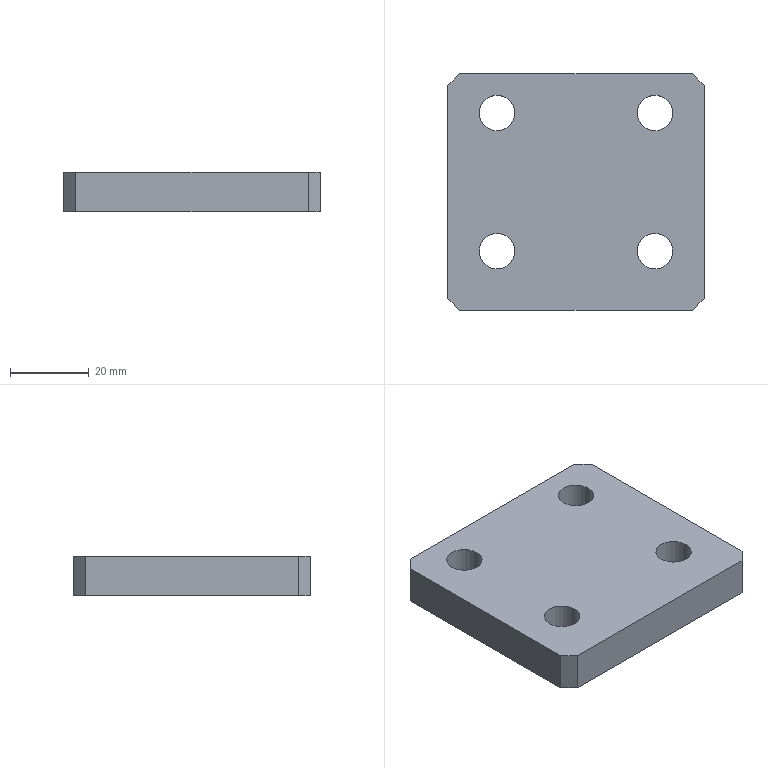Part | SolidWorks | features BaseBody 1 | 1 solid | 18 faces | box 65 x 60 x 10 mm | volume 36275 mm3 | plane 10 | cylinder 8 | commonest cylinder face diameters 9 x8
STEP:
#1=CARTESIAN_POINT('',(24.5,-15.,10.));
#2=VERTEX_POINT('',#1);
#3=CARTESIAN_POINT('',(15.5,-15.,10.));
#4=VERTEX_POINT('',#3);
#5=CARTESIAN_POINT('',(20.,-15.,10.));
#6=DIRECTION('',(0.,0.,-1.));
#7=DIRECTION('',(-1.,0.,0.));
#8=AXIS2_PLACEMENT_3D('',#5,#6,#7);
#9=CIRCLE('',#8,4.5);
#10=EDGE_CURVE('',#2,#4,#9,.T.);
#11=ORIENTED_EDGE('',*,*,#10,.F.);
#12=CARTESIAN_POINT('',(24.5,-15.,0.));
#13=VERTEX_POINT('',#12);
#14=CARTESIAN_POINT('',(24.5,-15.,0.));
#15=DIRECTION('',(0.,0.,-1.));
#16=VECTOR('',#15,1000.);
#17=LINE('',#14,#16);
#18=EDGE_CURVE('',#2,#13,#17,.T.);
#19=ORIENTED_EDGE('',*,*,#18,.T.);
#20=CARTESIAN_POINT('',(15.5,-15.,0.));
#21=VERTEX_POINT('',#20);
#22=CARTESIAN_POINT('',(20.,-15.,0.));
#23=DIRECTION('',(0.,0.,-1.));
#24=DIRECTION('',(-1.,0.,0.));
#25=AXIS2_PLACEMENT_3D('',#22,#23,#24);
#26=CIRCLE('',#25,4.5);
#27=EDGE_CURVE('',#13,#21,#26,.T.);
#28=ORIENTED_EDGE('',*,*,#27,.T.);
#29=CARTESIAN_POINT('',(15.5,-15.,0.));
#30=DIRECTION('',(0.,0.,-1.));
#31=VECTOR('',#30,1000.);
#32=LINE('',#29,#31);
#33=EDGE_CURVE('',#4,#21,#32,.T.);
#34=ORIENTED_EDGE('',*,*,#33,.F.);
#35=EDGE_LOOP('',(#11,#19,#28,#34));
#36=FACE_OUTER_BOUND('',#35,.T.);
#37=CARTESIAN_POINT('',(20.,-15.,0.));
#38=DIRECTION('',(0.,0.,-1.));
#39=DIRECTION('',(-1.,0.,0.));
#40=AXIS2_PLACEMENT_3D('',#37,#38,#39);
#41=CYLINDRICAL_SURFACE('',#40,4.5);
#42=ADVANCED_FACE('',(#36),#41,.F.);
#43=CARTESIAN_POINT('',(-15.5,-15.,10.));
#44=VERTEX_POINT('',#43);
#45=CARTESIAN_POINT('',(-24.5,-15.,10.));
#46=VERTEX_POINT('',#45);
#47=CARTESIAN_POINT('',(-20.,-15.,10.));
#48=DIRECTION('',(0.,0.,-1.));
#49=DIRECTION('',(-1.,0.,0.));
#50=AXIS2_PLACEMENT_3D('',#47,#48,#49);
#51=CIRCLE('',#50,4.5);
#52=EDGE_CURVE('',#44,#46,#51,.T.);
#53=ORIENTED_EDGE('',*,*,#52,.F.);
#54=CARTESIAN_POINT('',(-15.5,-15.,0.));
#55=VERTEX_POINT('',#54);
#56=CARTESIAN_POINT('',(-15.5,-15.,0.));
#57=DIRECTION('',(0.,0.,-1.));
#58=VECTOR('',#57,1000.);
#59=LINE('',#56,#58);
#60=EDGE_CURVE('',#44,#55,#59,.T.);
#61=ORIENTED_EDGE('',*,*,#60,.T.);
#62=CARTESIAN_POINT('',(-24.5,-15.,0.));
#63=VERTEX_POINT('',#62);
#64=CARTESIAN_POINT('',(-20.,-15.,0.));
#65=DIRECTION('',(0.,0.,-1.));
#66=DIRECTION('',(-1.,0.,0.));
#67=AXIS2_PLACEMENT_3D('',#64,#65,#66);
#68=CIRCLE('',#67,4.5);
#69=EDGE_CURVE('',#55,#63,#68,.T.);
#70=ORIENTED_EDGE('',*,*,#69,.T.);
#71=CARTESIAN_POINT('',(-24.5,-15.,0.));
#72=DIRECTION('',(0.,0.,-1.));
#73=VECTOR('',#72,1000.);
#74=LINE('',#71,#73);
#75=EDGE_CURVE('',#46,#63,#74,.T.);
#76=ORIENTED_EDGE('',*,*,#75,.F.);
#77=EDGE_LOOP('',(#53,#61,#70,#76));
#78=FACE_OUTER_BOUND('',#77,.T.);
#79=CARTESIAN_POINT('',(-20.,-15.,0.));
#80=DIRECTION('',(0.,0.,-1.));
#81=DIRECTION('',(-1.,0.,0.));
#82=AXIS2_PLACEMENT_3D('',#79,#80,#81);
#83=CYLINDRICAL_SURFACE('',#82,4.5);
#84=ADVANCED_FACE('',(#78),#83,.F.);
#85=CARTESIAN_POINT('',(24.5,20.,10.));
#86=VERTEX_POINT('',#85);
#87=CARTESIAN_POINT('',(15.5,20.,10.));
#88=VERTEX_POINT('',#87);
#89=CARTESIAN_POINT('',(20.,20.,10.));
#90=DIRECTION('',(0.,0.,-1.));
#91=DIRECTION('',(-1.,0.,0.));
#92=AXIS2_PLACEMENT_3D('',#89,#90,#91);
#93=CIRCLE('',#92,4.5);
#94=EDGE_CURVE('',#86,#88,#93,.T.);
#95=ORIENTED_EDGE('',*,*,#94,.F.);
#96=CARTESIAN_POINT('',(24.5,20.,0.));
#97=VERTEX_POINT('',#96);
#98=CARTESIAN_POINT('',(24.5,20.,0.));
#99=DIRECTION('',(0.,0.,-1.));
#100=VECTOR('',#99,1000.);
#101=LINE('',#98,#100);
#102=EDGE_CURVE('',#86,#97,#101,.T.);
#103=ORIENTED_EDGE('',*,*,#102,.T.);
#104=CARTESIAN_POINT('',(15.5,20.,0.));
#105=VERTEX_POINT('',#104);
#106=CARTESIAN_POINT('',(20.,20.,0.));
#107=DIRECTION('',(0.,0.,-1.));
#108=DIRECTION('',(-1.,0.,0.));
#109=AXIS2_PLACEMENT_3D('',#106,#107,#108);
#110=CIRCLE('',#109,4.5);
#111=EDGE_CURVE('',#97,#105,#110,.T.);
#112=ORIENTED_EDGE('',*,*,#111,.T.);
#113=CARTESIAN_POINT('',(15.5,20.,0.));
#114=DIRECTION('',(0.,0.,-1.));
#115=VECTOR('',#114,1000.);
#116=LINE('',#113,#115);
#117=EDGE_CURVE('',#88,#105,#116,.T.);
#118=ORIENTED_EDGE('',*,*,#117,.F.);
#119=EDGE_LOOP('',(#95,#103,#112,#118));
#120=FACE_OUTER_BOUND('',#119,.T.);
#121=CARTESIAN_POINT('',(20.,20.,0.));
#122=DIRECTION('',(0.,0.,-1.));
#123=DIRECTION('',(-1.,0.,0.));
#124=AXIS2_PLACEMENT_3D('',#121,#122,#123);
#125=CYLINDRICAL_SURFACE('',#124,4.5);
#126=ADVANCED_FACE('',(#120),#125,.F.);
#127=CARTESIAN_POINT('',(-15.5,20.,10.));
#128=VERTEX_POINT('',#127);
#129=CARTESIAN_POINT('',(-24.5,20.,10.));
#130=VERTEX_POINT('',#129);
#131=CARTESIAN_POINT('',(-20.,20.,10.));
#132=DIRECTION('',(0.,0.,-1.));
#133=DIRECTION('',(-1.,0.,0.));
#134=AXIS2_PLACEMENT_3D('',#131,#132,#133);
#135=CIRCLE('',#134,4.5);
#136=EDGE_CURVE('',#128,#130,#135,.T.);
#137=ORIENTED_EDGE('',*,*,#136,.F.);
#138=CARTESIAN_POINT('',(-15.5,20.,0.));
#139=VERTEX_POINT('',#138);
#140=CARTESIAN_POINT('',(-15.5,20.,0.));
#141=DIRECTION('',(0.,0.,-1.));
#142=VECTOR('',#141,1000.);
#143=LINE('',#140,#142);
#144=EDGE_CURVE('',#128,#139,#143,.T.);
#145=ORIENTED_EDGE('',*,*,#144,.T.);
#146=CARTESIAN_POINT('',(-24.5,20.,0.));
#147=VERTEX_POINT('',#146);
#148=CARTESIAN_POINT('',(-20.,20.,0.));
#149=DIRECTION('',(0.,0.,-1.));
#150=DIRECTION('',(-1.,0.,0.));
#151=AXIS2_PLACEMENT_3D('',#148,#149,#150);
#152=CIRCLE('',#151,4.5);
#153=EDGE_CURVE('',#139,#147,#152,.T.);
#154=ORIENTED_EDGE('',*,*,#153,.T.);
#155=CARTESIAN_POINT('',(-24.5,20.,0.));
#156=DIRECTION('',(0.,0.,-1.));
#157=VECTOR('',#156,1000.);
#158=LINE('',#155,#157);
#159=EDGE_CURVE('',#130,#147,#158,.T.);
#160=ORIENTED_EDGE('',*,*,#159,.F.);
#161=EDGE_LOOP('',(#137,#145,#154,#160));
#162=FACE_OUTER_BOUND('',#161,.T.);
#163=CARTESIAN_POINT('',(-20.,20.,0.));
#164=DIRECTION('',(0.,0.,-1.));
#165=DIRECTION('',(-1.,0.,0.));
#166=AXIS2_PLACEMENT_3D('',#163,#164,#165);
#167=CYLINDRICAL_SURFACE('',#166,4.5);
#168=ADVANCED_FACE('',(#162),#167,.F.);
#169=CARTESIAN_POINT('',(-32.5,27.,0.));
#170=VERTEX_POINT('',#169);
#171=CARTESIAN_POINT('',(-32.5,-27.,0.));
#172=VERTEX_POINT('',#171);
#173=CARTESIAN_POINT('',(-32.5,30.,0.));
#174=DIRECTION('',(0.,-1.,0.));
#175=VECTOR('',#174,1000.);
#176=LINE('',#173,#175);
#177=EDGE_CURVE('',#170,#172,#176,.T.);
#178=ORIENTED_EDGE('',*,*,#177,.T.);
#179=CARTESIAN_POINT('',(-32.5,-27.,10.));
#180=VERTEX_POINT('',#179);
#181=CARTESIAN_POINT('',(-32.5,-27.,10.));
#182=DIRECTION('',(0.,0.,1.));
#183=VECTOR('',#182,1000.);
#184=LINE('',#181,#183);
#185=EDGE_CURVE('',#172,#180,#184,.T.);
#186=ORIENTED_EDGE('',*,*,#185,.T.);
#187=CARTESIAN_POINT('',(-32.5,27.,10.));
#188=VERTEX_POINT('',#187);
#189=CARTESIAN_POINT('',(-32.5,30.,10.));
#190=DIRECTION('',(0.,-1.,0.));
#191=VECTOR('',#190,1000.);
#192=LINE('',#189,#191);
#193=EDGE_CURVE('',#188,#180,#192,.T.);
#194=ORIENTED_EDGE('',*,*,#193,.F.);
#195=CARTESIAN_POINT('',(-32.5,27.,10.));
#196=DIRECTION('',(0.,0.,-1.));
#197=VECTOR('',#196,1000.);
#198=LINE('',#195,#197);
#199=EDGE_CURVE('',#188,#170,#198,.T.);
#200=ORIENTED_EDGE('',*,*,#199,.T.);
#201=EDGE_LOOP('',(#178,#186,#194,#200));
#202=FACE_OUTER_BOUND('',#201,.T.);
#203=CARTESIAN_POINT('',(-32.5,30.,10.));
#204=DIRECTION('',(1.,0.,0.));
#205=DIRECTION('',(0.,1.,0.));
#206=AXIS2_PLACEMENT_3D('',#203,#204,#205);
#207=PLANE('',#206);
#208=ADVANCED_FACE('',(#202),#207,.F.);
#209=CARTESIAN_POINT('',(-29.5,-30.,10.));
#210=VERTEX_POINT('',#209);
#211=CARTESIAN_POINT('',(29.5,-30.,10.));
#212=VERTEX_POINT('',#211);
#213=CARTESIAN_POINT('',(32.5,-30.,10.));
#214=DIRECTION('',(1.,0.,0.));
#215=VECTOR('',#214,1000.);
#216=LINE('',#213,#215);
#217=EDGE_CURVE('',#210,#212,#216,.T.);
#218=ORIENTED_EDGE('',*,*,#217,.F.);
#219=CARTESIAN_POINT('',(-29.5,-30.,0.));
#220=VERTEX_POINT('',#219);
#221=CARTESIAN_POINT('',(-29.5,-30.,10.));
#222=DIRECTION('',(0.,0.,-1.));
#223=VECTOR('',#222,1000.);
#224=LINE('',#221,#223);
#225=EDGE_CURVE('',#210,#220,#224,.T.);
#226=ORIENTED_EDGE('',*,*,#225,.T.);
#227=CARTESIAN_POINT('',(29.5,-30.,0.));
#228=VERTEX_POINT('',#227);
#229=CARTESIAN_POINT('',(32.5,-30.,0.));
#230=DIRECTION('',(1.,0.,0.));
#231=VECTOR('',#230,1000.);
#232=LINE('',#229,#231);
#233=EDGE_CURVE('',#220,#228,#232,.T.);
#234=ORIENTED_EDGE('',*,*,#233,.T.);
#235=CARTESIAN_POINT('',(29.5,-30.,10.));
#236=DIRECTION('',(0.,0.,1.));
#237=VECTOR('',#236,1000.);
#238=LINE('',#235,#237);
#239=EDGE_CURVE('',#228,#212,#238,.T.);
#240=ORIENTED_EDGE('',*,*,#239,.T.);
#241=EDGE_LOOP('',(#218,#226,#234,#240));
#242=FACE_OUTER_BOUND('',#241,.T.);
#243=CARTESIAN_POINT('',(32.5,-30.,10.));
#244=DIRECTION('',(0.,1.,0.));
#245=DIRECTION('',(-1.,0.,0.));
#246=AXIS2_PLACEMENT_3D('',#243,#244,#245);
#247=PLANE('',#246);
#248=ADVANCED_FACE('',(#242),#247,.F.);
#249=CARTESIAN_POINT('',(32.5,-27.,10.));
#250=VERTEX_POINT('',#249);
#251=CARTESIAN_POINT('',(32.5,27.,10.));
#252=VERTEX_POINT('',#251);
#253=CARTESIAN_POINT('',(32.5,30.,10.));
#254=DIRECTION('',(0.,1.,0.));
#255=VECTOR('',#254,1000.);
#256=LINE('',#253,#255);
#257=EDGE_CURVE('',#250,#252,#256,.T.);
#258=ORIENTED_EDGE('',*,*,#257,.F.);
#259=CARTESIAN_POINT('',(32.5,-27.,0.));
#260=VERTEX_POINT('',#259);
#261=CARTESIAN_POINT('',(32.5,-27.,10.));
#262=DIRECTION('',(0.,0.,-1.));
#263=VECTOR('',#262,1000.);
#264=LINE('',#261,#263);
#265=EDGE_CURVE('',#250,#260,#264,.T.);
#266=ORIENTED_EDGE('',*,*,#265,.T.);
#267=CARTESIAN_POINT('',(32.5,27.,0.));
#268=VERTEX_POINT('',#267);
#269=CARTESIAN_POINT('',(32.5,30.,0.));
#270=DIRECTION('',(0.,1.,0.));
#271=VECTOR('',#270,1000.);
#272=LINE('',#269,#271);
#273=EDGE_CURVE('',#260,#268,#272,.T.);
#274=ORIENTED_EDGE('',*,*,#273,.T.);
#275=CARTESIAN_POINT('',(32.5,27.,10.));
#276=DIRECTION('',(0.,0.,1.));
#277=VECTOR('',#276,1000.);
#278=LINE('',#275,#277);
#279=EDGE_CURVE('',#268,#252,#278,.T.);
#280=ORIENTED_EDGE('',*,*,#279,.T.);
#281=EDGE_LOOP('',(#258,#266,#274,#280));
#282=FACE_OUTER_BOUND('',#281,.T.);
#283=CARTESIAN_POINT('',(32.5,30.,10.));
#284=DIRECTION('',(-1.,0.,0.));
#285=DIRECTION('',(0.,-1.,0.));
#286=AXIS2_PLACEMENT_3D('',#283,#284,#285);
#287=PLANE('',#286);
#288=ADVANCED_FACE('',(#282),#287,.F.);
#289=CARTESIAN_POINT('',(29.5,30.,0.));
#290=VERTEX_POINT('',#289);
#291=CARTESIAN_POINT('',(-29.5,30.,0.));
#292=VERTEX_POINT('',#291);
#293=CARTESIAN_POINT('',(32.5,30.,0.));
#294=DIRECTION('',(-1.,0.,0.));
#295=VECTOR('',#294,1000.);
#296=LINE('',#293,#295);
#297=EDGE_CURVE('',#290,#292,#296,.T.);
#298=ORIENTED_EDGE('',*,*,#297,.T.);
#299=CARTESIAN_POINT('',(-29.5,30.,10.));
#300=VERTEX_POINT('',#299);
#301=CARTESIAN_POINT('',(-29.5,30.,10.));
#302=DIRECTION('',(0.,0.,1.));
#303=VECTOR('',#302,1000.);
#304=LINE('',#301,#303);
#305=EDGE_CURVE('',#292,#300,#304,.T.);
#306=ORIENTED_EDGE('',*,*,#305,.T.);
#307=CARTESIAN_POINT('',(29.5,30.,10.));
#308=VERTEX_POINT('',#307);
#309=CARTESIAN_POINT('',(32.5,30.,10.));
#310=DIRECTION('',(-1.,0.,0.));
#311=VECTOR('',#310,1000.);
#312=LINE('',#309,#311);
#313=EDGE_CURVE('',#308,#300,#312,.T.);
#314=ORIENTED_EDGE('',*,*,#313,.F.);
#315=CARTESIAN_POINT('',(29.5,30.,10.));
#316=DIRECTION('',(0.,0.,-1.));
#317=VECTOR('',#316,1000.);
#318=LINE('',#315,#317);
#319=EDGE_CURVE('',#308,#290,#318,.T.);
#320=ORIENTED_EDGE('',*,*,#319,.T.);
#321=EDGE_LOOP('',(#298,#306,#314,#320));
#322=FACE_OUTER_BOUND('',#321,.T.);
#323=CARTESIAN_POINT('',(32.5,30.,10.));
#324=DIRECTION('',(0.,-1.,0.));
#325=DIRECTION('',(1.,0.,0.));
#326=AXIS2_PLACEMENT_3D('',#323,#324,#325);
#327=PLANE('',#326);
#328=ADVANCED_FACE('',(#322),#327,.F.);
#329=CARTESIAN_POINT('',(20.,-15.,10.));
#330=DIRECTION('',(0.,0.,-1.));
#331=DIRECTION('',(-1.,0.,0.));
#332=AXIS2_PLACEMENT_3D('',#329,#330,#331);
#333=CIRCLE('',#332,4.5);
#334=EDGE_CURVE('',#4,#2,#333,.T.);
#335=ORIENTED_EDGE('',*,*,#334,.T.);
#336=ORIENTED_EDGE('',*,*,#10,.T.);
#337=EDGE_LOOP('',(#335,#336));
#338=FACE_BOUND('',#337,.T.);
#339=CARTESIAN_POINT('',(-20.,-15.,10.));
#340=DIRECTION('',(0.,0.,-1.));
#341=DIRECTION('',(-1.,0.,0.));
#342=AXIS2_PLACEMENT_3D('',#339,#340,#341);
#343=CIRCLE('',#342,4.5);
#344=EDGE_CURVE('',#46,#44,#343,.T.);
#345=ORIENTED_EDGE('',*,*,#344,.T.);
#346=ORIENTED_EDGE('',*,*,#52,.T.);
#347=EDGE_LOOP('',(#345,#346));
#348=FACE_BOUND('',#347,.T.);
#349=CARTESIAN_POINT('',(20.,20.,10.));
#350=DIRECTION('',(0.,0.,-1.));
#351=DIRECTION('',(-1.,0.,0.));
#352=AXIS2_PLACEMENT_3D('',#349,#350,#351);
#353=CIRCLE('',#352,4.5);
#354=EDGE_CURVE('',#88,#86,#353,.T.);
#355=ORIENTED_EDGE('',*,*,#354,.T.);
#356=ORIENTED_EDGE('',*,*,#94,.T.);
#357=EDGE_LOOP('',(#355,#356));
#358=FACE_BOUND('',#357,.T.);
#359=CARTESIAN_POINT('',(-20.,20.,10.));
#360=DIRECTION('',(0.,0.,-1.));
#361=DIRECTION('',(-1.,0.,0.));
#362=AXIS2_PLACEMENT_3D('',#359,#360,#361);
#363=CIRCLE('',#362,4.5);
#364=EDGE_CURVE('',#130,#128,#363,.T.);
#365=ORIENTED_EDGE('',*,*,#364,.T.);
#366=ORIENTED_EDGE('',*,*,#136,.T.);
#367=EDGE_LOOP('',(#365,#366));
#368=FACE_BOUND('',#367,.T.);
#369=ORIENTED_EDGE('',*,*,#193,.T.);
#370=CARTESIAN_POINT('',(-29.5,-30.,10.));
#371=DIRECTION('',(0.7071,-0.7071,0.));
#372=VECTOR('',#371,1000.);
#373=LINE('',#370,#372);
#374=EDGE_CURVE('',#180,#210,#373,.T.);
#375=ORIENTED_EDGE('',*,*,#374,.T.);
#376=ORIENTED_EDGE('',*,*,#217,.T.);
#377=CARTESIAN_POINT('',(32.5,-27.,10.));
#378=DIRECTION('',(0.7071,0.7071,0.));
#379=VECTOR('',#378,1000.);
#380=LINE('',#377,#379);
#381=EDGE_CURVE('',#212,#250,#380,.T.);
#382=ORIENTED_EDGE('',*,*,#381,.T.);
#383=ORIENTED_EDGE('',*,*,#257,.T.);
#384=CARTESIAN_POINT('',(29.5,30.,10.));
#385=DIRECTION('',(-0.7071,0.7071,0.));
#386=VECTOR('',#385,1000.);
#387=LINE('',#384,#386);
#388=EDGE_CURVE('',#252,#308,#387,.T.);
#389=ORIENTED_EDGE('',*,*,#388,.T.);
#390=ORIENTED_EDGE('',*,*,#313,.T.);
#391=CARTESIAN_POINT('',(-32.5,27.,10.));
#392=DIRECTION('',(-0.7071,-0.7071,0.));
#393=VECTOR('',#392,1000.);
#394=LINE('',#391,#393);
#395=EDGE_CURVE('',#300,#188,#394,.T.);
#396=ORIENTED_EDGE('',*,*,#395,.T.);
#397=EDGE_LOOP('',(#369,#375,#376,#382,#383,#389,#390,#396));
#398=FACE_OUTER_BOUND('',#397,.T.);
#399=CARTESIAN_POINT('',(0.,0.,10.));
#400=DIRECTION('',(0.,0.,-1.));
#401=DIRECTION('',(-1.,0.,0.));
#402=AXIS2_PLACEMENT_3D('',#399,#400,#401);
#403=PLANE('',#402);
#404=ADVANCED_FACE('',(#338,#348,#358,#368,#398),#403,.F.);
#405=CARTESIAN_POINT('',(20.,-15.,0.));
#406=DIRECTION('',(0.,0.,-1.));
#407=DIRECTION('',(-1.,0.,0.));
#408=AXIS2_PLACEMENT_3D('',#405,#406,#407);
#409=CIRCLE('',#408,4.5);
#410=EDGE_CURVE('',#21,#13,#409,.T.);
#411=ORIENTED_EDGE('',*,*,#410,.F.);
#412=ORIENTED_EDGE('',*,*,#27,.F.);
#413=EDGE_LOOP('',(#411,#412));
#414=FACE_BOUND('',#413,.T.);
#415=CARTESIAN_POINT('',(-20.,-15.,0.));
#416=DIRECTION('',(0.,0.,-1.));
#417=DIRECTION('',(-1.,0.,0.));
#418=AXIS2_PLACEMENT_3D('',#415,#416,#417);
#419=CIRCLE('',#418,4.5);
#420=EDGE_CURVE('',#63,#55,#419,.T.);
#421=ORIENTED_EDGE('',*,*,#420,.F.);
#422=ORIENTED_EDGE('',*,*,#69,.F.);
#423=EDGE_LOOP('',(#421,#422));
#424=FACE_BOUND('',#423,.T.);
#425=CARTESIAN_POINT('',(20.,20.,0.));
#426=DIRECTION('',(0.,0.,-1.));
#427=DIRECTION('',(-1.,0.,0.));
#428=AXIS2_PLACEMENT_3D('',#425,#426,#427);
#429=CIRCLE('',#428,4.5);
#430=EDGE_CURVE('',#105,#97,#429,.T.);
#431=ORIENTED_EDGE('',*,*,#430,.F.);
#432=ORIENTED_EDGE('',*,*,#111,.F.);
#433=EDGE_LOOP('',(#431,#432));
#434=FACE_BOUND('',#433,.T.);
#435=CARTESIAN_POINT('',(-20.,20.,0.));
#436=DIRECTION('',(0.,0.,-1.));
#437=DIRECTION('',(-1.,0.,0.));
#438=AXIS2_PLACEMENT_3D('',#435,#436,#437);
#439=CIRCLE('',#438,4.5);
#440=EDGE_CURVE('',#147,#139,#439,.T.);
#441=ORIENTED_EDGE('',*,*,#440,.F.);
#442=ORIENTED_EDGE('',*,*,#153,.F.);
#443=EDGE_LOOP('',(#441,#442));
#444=FACE_BOUND('',#443,.T.);
#445=ORIENTED_EDGE('',*,*,#233,.F.);
#446=CARTESIAN_POINT('',(-29.75,-29.75,0.));
#447=DIRECTION('',(-0.7071,0.7071,0.));
#448=VECTOR('',#447,1000.);
#449=LINE('',#446,#448);
#450=EDGE_CURVE('',#220,#172,#449,.T.);
#451=ORIENTED_EDGE('',*,*,#450,.T.);
#452=ORIENTED_EDGE('',*,*,#177,.F.);
#453=CARTESIAN_POINT('',(-29.75,29.75,0.));
#454=DIRECTION('',(0.7071,0.7071,0.));
#455=VECTOR('',#454,1000.);
#456=LINE('',#453,#455);
#457=EDGE_CURVE('',#170,#292,#456,.T.);
#458=ORIENTED_EDGE('',*,*,#457,.T.);
#459=ORIENTED_EDGE('',*,*,#297,.F.);
#460=CARTESIAN_POINT('',(29.75,29.75,0.));
#461=DIRECTION('',(0.7071,-0.7071,0.));
#462=VECTOR('',#461,1000.);
#463=LINE('',#460,#462);
#464=EDGE_CURVE('',#290,#268,#463,.T.);
#465=ORIENTED_EDGE('',*,*,#464,.T.);
#466=ORIENTED_EDGE('',*,*,#273,.F.);
#467=CARTESIAN_POINT('',(29.75,-29.75,0.));
#468=DIRECTION('',(-0.7071,-0.7071,0.));
#469=VECTOR('',#468,1000.);
#470=LINE('',#467,#469);
#471=EDGE_CURVE('',#260,#228,#470,.T.);
#472=ORIENTED_EDGE('',*,*,#471,.T.);
#473=EDGE_LOOP('',(#445,#451,#452,#458,#459,#465,#466,#472));
#474=FACE_OUTER_BOUND('',#473,.T.);
#475=CARTESIAN_POINT('',(0.,0.,0.));
#476=DIRECTION('',(0.,0.,-1.));
#477=DIRECTION('',(-1.,0.,0.));
#478=AXIS2_PLACEMENT_3D('',#475,#476,#477);
#479=PLANE('',#478);
#480=ADVANCED_FACE('',(#414,#424,#434,#444,#474),#479,.T.);
#481=ORIENTED_EDGE('',*,*,#144,.F.);
#482=ORIENTED_EDGE('',*,*,#364,.F.);
#483=ORIENTED_EDGE('',*,*,#159,.T.);
#484=ORIENTED_EDGE('',*,*,#440,.T.);
#485=EDGE_LOOP('',(#481,#482,#483,#484));
#486=FACE_OUTER_BOUND('',#485,.T.);
#487=CARTESIAN_POINT('',(-20.,20.,0.));
#488=DIRECTION('',(0.,0.,-1.));
#489=DIRECTION('',(-1.,0.,0.));
#490=AXIS2_PLACEMENT_3D('',#487,#488,#489);
#491=CYLINDRICAL_SURFACE('',#490,4.5);
#492=ADVANCED_FACE('',(#486),#491,.F.);
#493=ORIENTED_EDGE('',*,*,#102,.F.);
#494=ORIENTED_EDGE('',*,*,#354,.F.);
#495=ORIENTED_EDGE('',*,*,#117,.T.);
#496=ORIENTED_EDGE('',*,*,#430,.T.);
#497=EDGE_LOOP('',(#493,#494,#495,#496));
#498=FACE_OUTER_BOUND('',#497,.T.);
#499=CARTESIAN_POINT('',(20.,20.,0.));
#500=DIRECTION('',(0.,0.,-1.));
#501=DIRECTION('',(-1.,0.,0.));
#502=AXIS2_PLACEMENT_3D('',#499,#500,#501);
#503=CYLINDRICAL_SURFACE('',#502,4.5);
#504=ADVANCED_FACE('',(#498),#503,.F.);
#505=ORIENTED_EDGE('',*,*,#60,.F.);
#506=ORIENTED_EDGE('',*,*,#344,.F.);
#507=ORIENTED_EDGE('',*,*,#75,.T.);
#508=ORIENTED_EDGE('',*,*,#420,.T.);
#509=EDGE_LOOP('',(#505,#506,#507,#508));
#510=FACE_OUTER_BOUND('',#509,.T.);
#511=CARTESIAN_POINT('',(-20.,-15.,0.));
#512=DIRECTION('',(0.,0.,-1.));
#513=DIRECTION('',(-1.,0.,0.));
#514=AXIS2_PLACEMENT_3D('',#511,#512,#513);
#515=CYLINDRICAL_SURFACE('',#514,4.5);
#516=ADVANCED_FACE('',(#510),#515,.F.);
#517=ORIENTED_EDGE('',*,*,#18,.F.);
#518=ORIENTED_EDGE('',*,*,#334,.F.);
#519=ORIENTED_EDGE('',*,*,#33,.T.);
#520=ORIENTED_EDGE('',*,*,#410,.T.);
#521=EDGE_LOOP('',(#517,#518,#519,#520));
#522=FACE_OUTER_BOUND('',#521,.T.);
#523=CARTESIAN_POINT('',(20.,-15.,0.));
#524=DIRECTION('',(0.,0.,-1.));
#525=DIRECTION('',(-1.,0.,0.));
#526=AXIS2_PLACEMENT_3D('',#523,#524,#525);
#527=CYLINDRICAL_SURFACE('',#526,4.5);
#528=ADVANCED_FACE('',(#522),#527,.F.);
#529=ORIENTED_EDGE('',*,*,#374,.F.);
#530=ORIENTED_EDGE('',*,*,#185,.F.);
#531=ORIENTED_EDGE('',*,*,#450,.F.);
#532=ORIENTED_EDGE('',*,*,#225,.F.);
#533=EDGE_LOOP('',(#529,#530,#531,#532));
#534=FACE_OUTER_BOUND('',#533,.T.);
#535=CARTESIAN_POINT('',(-29.5,-30.,10.));
#536=DIRECTION('',(0.7071,0.7071,0.));
#537=DIRECTION('',(0.,0.,-1.));
#538=AXIS2_PLACEMENT_3D('',#535,#536,#537);
#539=PLANE('',#538);
#540=ADVANCED_FACE('',(#534),#539,.F.);
#541=ORIENTED_EDGE('',*,*,#381,.F.);
#542=ORIENTED_EDGE('',*,*,#239,.F.);
#543=ORIENTED_EDGE('',*,*,#471,.F.);
#544=ORIENTED_EDGE('',*,*,#265,.F.);
#545=EDGE_LOOP('',(#541,#542,#543,#544));
#546=FACE_OUTER_BOUND('',#545,.T.);
#547=CARTESIAN_POINT('',(32.5,-27.,10.));
#548=DIRECTION('',(-0.7071,0.7071,0.));
#549=DIRECTION('',(0.,0.,-1.));
#550=AXIS2_PLACEMENT_3D('',#547,#548,#549);
#551=PLANE('',#550);
#552=ADVANCED_FACE('',(#546),#551,.F.);
#553=ORIENTED_EDGE('',*,*,#395,.F.);
#554=ORIENTED_EDGE('',*,*,#305,.F.);
#555=ORIENTED_EDGE('',*,*,#457,.F.);
#556=ORIENTED_EDGE('',*,*,#199,.F.);
#557=EDGE_LOOP('',(#553,#554,#555,#556));
#558=FACE_OUTER_BOUND('',#557,.T.);
#559=CARTESIAN_POINT('',(-32.5,27.,10.));
#560=DIRECTION('',(0.7071,-0.7071,0.));
#561=DIRECTION('',(0.,0.,-1.));
#562=AXIS2_PLACEMENT_3D('',#559,#560,#561);
#563=PLANE('',#562);
#564=ADVANCED_FACE('',(#558),#563,.F.);
#565=ORIENTED_EDGE('',*,*,#388,.F.);
#566=ORIENTED_EDGE('',*,*,#279,.F.);
#567=ORIENTED_EDGE('',*,*,#464,.F.);
#568=ORIENTED_EDGE('',*,*,#319,.F.);
#569=EDGE_LOOP('',(#565,#566,#567,#568));
#570=FACE_OUTER_BOUND('',#569,.T.);
#571=CARTESIAN_POINT('',(29.5,30.,10.));
#572=DIRECTION('',(-0.7071,-0.7071,0.));
#573=DIRECTION('',(0.,0.,-1.));
#574=AXIS2_PLACEMENT_3D('',#571,#572,#573);
#575=PLANE('',#574);
#576=ADVANCED_FACE('',(#570),#575,.F.);
#577=CLOSED_SHELL('',(#42,#84,#126,#168,#208,#248,#288,#328,#404,#480,#492,#504,#516,#528,#540,#552,#564,#576));
#578=MANIFOLD_SOLID_BREP('',#577);
#579=CARTESIAN_POINT('',(0.,0.,0.));
#580=DIRECTION('',(0.,0.,1.));
#581=DIRECTION('',(1.,0.,0.));
#582=AXIS2_PLACEMENT_3D('',#579,#580,#581);
#583=(LENGTH_UNIT()NAMED_UNIT(*)SI_UNIT(.MILLI.,.METRE.));
#584=UNCERTAINTY_MEASURE_WITH_UNIT(LENGTH_MEASURE(0.00001),#583,'','');
#585=(NAMED_UNIT(*)PLANE_ANGLE_UNIT()SI_UNIT($,.RADIAN.));
#586=(NAMED_UNIT(*)SI_UNIT($,.STERADIAN.)SOLID_ANGLE_UNIT());
#587=(GEOMETRIC_REPRESENTATION_CONTEXT(3)GLOBAL_UNCERTAINTY_ASSIGNED_CONTEXT((#584))GLOBAL_UNIT_ASSIGNED_CONTEXT((#583,#585,#586))REPRESENTATION_CONTEXT('',''));
#588=ADVANCED_BREP_SHAPE_REPRESENTATION('',(#578,#582),#587);